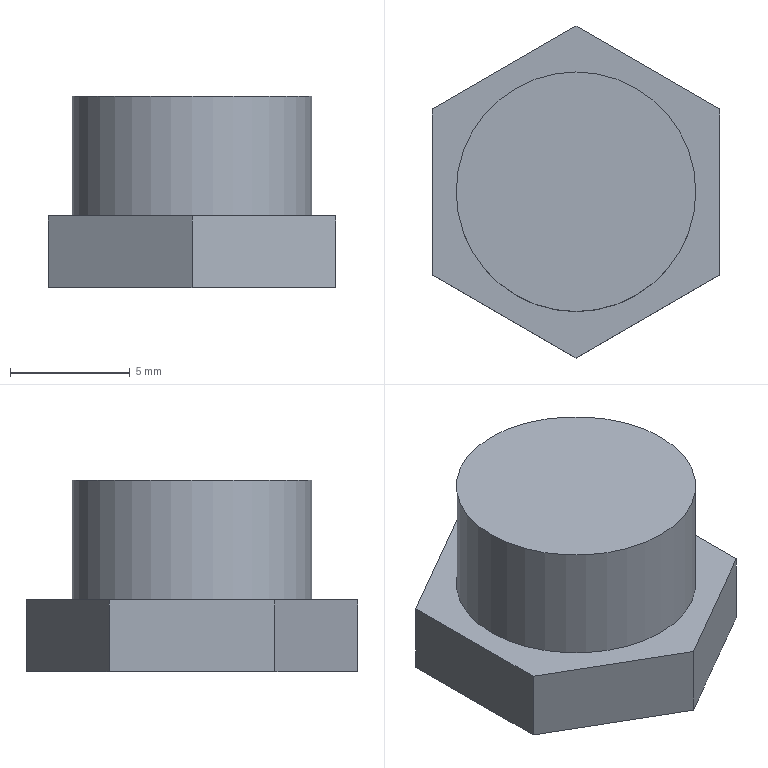Part | STEP file | 1-65.2 | 1 solid | 10 faces | box 12 x 13.856 x 8 mm | volume 766.822 mm3 | plane 9 | cylinder 1 | commonest cylinder face diameters 10 x1
STEP:
#1=CARTESIAN_POINT('',(0.,0.,0.));
#2=DIRECTION('',(0.,0.,1.));
#3=DIRECTION('',(1.,0.,0.));
#4=AXIS2_PLACEMENT_3D('',#1,#2,#3);
#5=CARTESIAN_POINT('',(-6.,-3.464,-3.));
#6=VERTEX_POINT('',#5);
#7=CARTESIAN_POINT('',(-6.,3.464,-3.));
#8=VERTEX_POINT('',#7);
#9=CARTESIAN_POINT('',(-6.,-3.464,-3.));
#10=DIRECTION('',(0.,1.,0.));
#11=VECTOR('',#10,1.);
#12=LINE('',#9,#11);
#13=CARTESIAN_POINT('',(0.9282,0.,-3.));
#14=DIRECTION('',(0.,0.,-1.));
#15=DIRECTION('',(1.,0.,0.));
#16=AXIS2_PLACEMENT_3D('',#13,#14,#15);
#17=PLANE('',#16);
#18=CARTESIAN_POINT('',(-6.928,3.464));
#19=DIRECTION('',(0.,-1.));
#20=VECTOR('',#19,1.);
#21=LINE('',#18,#20);
#22=(GEOMETRIC_REPRESENTATION_CONTEXT(2)PARAMETRIC_REPRESENTATION_CONTEXT()REPRESENTATION_CONTEXT('',''));
#23=DEFINITIONAL_REPRESENTATION('',(#21),#22);
#24=PCURVE('',#17,#23);
#25=CARTESIAN_POINT('',(-6.,0.,-1.5));
#26=DIRECTION('',(-1.,0.,0.));
#27=DIRECTION('',(0.,1.,0.));
#28=AXIS2_PLACEMENT_3D('',#25,#26,#27);
#29=PLANE('',#28);
#30=CARTESIAN_POINT('',(-3.464,1.5));
#31=DIRECTION('',(1.,0.));
#32=VECTOR('',#31,1.);
#33=LINE('',#30,#32);
#34=(GEOMETRIC_REPRESENTATION_CONTEXT(2)PARAMETRIC_REPRESENTATION_CONTEXT()REPRESENTATION_CONTEXT('',''));
#35=DEFINITIONAL_REPRESENTATION('',(#33),#34);
#36=PCURVE('',#29,#35);
#37=SURFACE_CURVE('',#12,(#24,#36),.PCURVE_S1.);
#38=EDGE_CURVE('',#6,#8,#37,.T.);
#39=ORIENTED_EDGE('',*,*,#38,.T.);
#40=CARTESIAN_POINT('',(0.,6.928,-3.));
#41=VERTEX_POINT('',#40);
#42=CARTESIAN_POINT('',(-6.,3.464,-3.));
#43=DIRECTION('',(0.866,0.5,0.));
#44=VECTOR('',#43,1.);
#45=LINE('',#42,#44);
#46=CARTESIAN_POINT('',(-6.928,-3.464));
#47=DIRECTION('',(0.866,-0.5));
#48=VECTOR('',#47,1.);
#49=LINE('',#46,#48);
#50=(GEOMETRIC_REPRESENTATION_CONTEXT(2)PARAMETRIC_REPRESENTATION_CONTEXT()REPRESENTATION_CONTEXT('',''));
#51=DEFINITIONAL_REPRESENTATION('',(#49),#50);
#52=PCURVE('',#17,#51);
#53=CARTESIAN_POINT('',(-3.,5.196,-1.5));
#54=DIRECTION('',(-0.5,0.866,0.));
#55=DIRECTION('',(0.866,0.5,0.));
#56=AXIS2_PLACEMENT_3D('',#53,#54,#55);
#57=PLANE('',#56);
#58=CARTESIAN_POINT('',(-3.464,1.5));
#59=DIRECTION('',(1.,0.));
#60=VECTOR('',#59,1.);
#61=LINE('',#58,#60);
#62=(GEOMETRIC_REPRESENTATION_CONTEXT(2)PARAMETRIC_REPRESENTATION_CONTEXT()REPRESENTATION_CONTEXT('',''));
#63=DEFINITIONAL_REPRESENTATION('',(#61),#62);
#64=PCURVE('',#57,#63);
#65=SURFACE_CURVE('',#45,(#52,#64),.PCURVE_S1.);
#66=EDGE_CURVE('',#8,#41,#65,.T.);
#67=ORIENTED_EDGE('',*,*,#66,.T.);
#68=CARTESIAN_POINT('',(6.,3.464,-3.));
#69=VERTEX_POINT('',#68);
#70=CARTESIAN_POINT('',(0.,6.928,-3.));
#71=DIRECTION('',(0.866,-0.5,0.));
#72=VECTOR('',#71,1.);
#73=LINE('',#70,#72);
#74=CARTESIAN_POINT('',(-0.9282,-6.928));
#75=DIRECTION('',(0.866,0.5));
#76=VECTOR('',#75,1.);
#77=LINE('',#74,#76);
#78=(GEOMETRIC_REPRESENTATION_CONTEXT(2)PARAMETRIC_REPRESENTATION_CONTEXT()REPRESENTATION_CONTEXT('',''));
#79=DEFINITIONAL_REPRESENTATION('',(#77),#78);
#80=PCURVE('',#17,#79);
#81=CARTESIAN_POINT('',(3.,5.196,-1.5));
#82=DIRECTION('',(0.5,0.866,0.));
#83=DIRECTION('',(0.866,-0.5,0.));
#84=AXIS2_PLACEMENT_3D('',#81,#82,#83);
#85=PLANE('',#84);
#86=CARTESIAN_POINT('',(-3.464,1.5));
#87=DIRECTION('',(1.,0.));
#88=VECTOR('',#87,1.);
#89=LINE('',#86,#88);
#90=(GEOMETRIC_REPRESENTATION_CONTEXT(2)PARAMETRIC_REPRESENTATION_CONTEXT()REPRESENTATION_CONTEXT('',''));
#91=DEFINITIONAL_REPRESENTATION('',(#89),#90);
#92=PCURVE('',#85,#91);
#93=SURFACE_CURVE('',#73,(#80,#92),.PCURVE_S1.);
#94=EDGE_CURVE('',#41,#69,#93,.T.);
#95=ORIENTED_EDGE('',*,*,#94,.T.);
#96=CARTESIAN_POINT('',(6.,-3.464,-3.));
#97=VERTEX_POINT('',#96);
#98=CARTESIAN_POINT('',(6.,3.464,-3.));
#99=DIRECTION('',(0.,-1.,0.));
#100=VECTOR('',#99,1.);
#101=LINE('',#98,#100);
#102=CARTESIAN_POINT('',(5.072,-3.464));
#103=DIRECTION('',(0.,1.));
#104=VECTOR('',#103,1.);
#105=LINE('',#102,#104);
#106=(GEOMETRIC_REPRESENTATION_CONTEXT(2)PARAMETRIC_REPRESENTATION_CONTEXT()REPRESENTATION_CONTEXT('',''));
#107=DEFINITIONAL_REPRESENTATION('',(#105),#106);
#108=PCURVE('',#17,#107);
#109=CARTESIAN_POINT('',(6.,0.,-1.5));
#110=DIRECTION('',(1.,0.,0.));
#111=DIRECTION('',(0.,-1.,0.));
#112=AXIS2_PLACEMENT_3D('',#109,#110,#111);
#113=PLANE('',#112);
#114=CARTESIAN_POINT('',(-3.464,1.5));
#115=DIRECTION('',(1.,0.));
#116=VECTOR('',#115,1.);
#117=LINE('',#114,#116);
#118=(GEOMETRIC_REPRESENTATION_CONTEXT(2)PARAMETRIC_REPRESENTATION_CONTEXT()REPRESENTATION_CONTEXT('',''));
#119=DEFINITIONAL_REPRESENTATION('',(#117),#118);
#120=PCURVE('',#113,#119);
#121=SURFACE_CURVE('',#101,(#108,#120),.PCURVE_S1.);
#122=EDGE_CURVE('',#69,#97,#121,.T.);
#123=ORIENTED_EDGE('',*,*,#122,.T.);
#124=CARTESIAN_POINT('',(0.,-6.928,-3.));
#125=VERTEX_POINT('',#124);
#126=CARTESIAN_POINT('',(6.,-3.464,-3.));
#127=DIRECTION('',(-0.866,-0.5,0.));
#128=VECTOR('',#127,1.);
#129=LINE('',#126,#128);
#130=CARTESIAN_POINT('',(5.072,3.464));
#131=DIRECTION('',(-0.866,0.5));
#132=VECTOR('',#131,1.);
#133=LINE('',#130,#132);
#134=(GEOMETRIC_REPRESENTATION_CONTEXT(2)PARAMETRIC_REPRESENTATION_CONTEXT()REPRESENTATION_CONTEXT('',''));
#135=DEFINITIONAL_REPRESENTATION('',(#133),#134);
#136=PCURVE('',#17,#135);
#137=CARTESIAN_POINT('',(3.,-5.196,-1.5));
#138=DIRECTION('',(0.5,-0.866,0.));
#139=DIRECTION('',(-0.866,-0.5,0.));
#140=AXIS2_PLACEMENT_3D('',#137,#138,#139);
#141=PLANE('',#140);
#142=CARTESIAN_POINT('',(-3.464,1.5));
#143=DIRECTION('',(1.,0.));
#144=VECTOR('',#143,1.);
#145=LINE('',#142,#144);
#146=(GEOMETRIC_REPRESENTATION_CONTEXT(2)PARAMETRIC_REPRESENTATION_CONTEXT()REPRESENTATION_CONTEXT('',''));
#147=DEFINITIONAL_REPRESENTATION('',(#145),#146);
#148=PCURVE('',#141,#147);
#149=SURFACE_CURVE('',#129,(#136,#148),.PCURVE_S1.);
#150=EDGE_CURVE('',#97,#125,#149,.T.);
#151=ORIENTED_EDGE('',*,*,#150,.T.);
#152=CARTESIAN_POINT('',(0.,-6.928,-3.));
#153=DIRECTION('',(-0.866,0.5,0.));
#154=VECTOR('',#153,1.);
#155=LINE('',#152,#154);
#156=CARTESIAN_POINT('',(-0.9282,6.928));
#157=DIRECTION('',(-0.866,-0.5));
#158=VECTOR('',#157,1.);
#159=LINE('',#156,#158);
#160=(GEOMETRIC_REPRESENTATION_CONTEXT(2)PARAMETRIC_REPRESENTATION_CONTEXT()REPRESENTATION_CONTEXT('',''));
#161=DEFINITIONAL_REPRESENTATION('',(#159),#160);
#162=PCURVE('',#17,#161);
#163=CARTESIAN_POINT('',(-3.,-5.196,-1.5));
#164=DIRECTION('',(-0.5,-0.866,0.));
#165=DIRECTION('',(-0.866,0.5,0.));
#166=AXIS2_PLACEMENT_3D('',#163,#164,#165);
#167=PLANE('',#166);
#168=CARTESIAN_POINT('',(-3.464,1.5));
#169=DIRECTION('',(1.,0.));
#170=VECTOR('',#169,1.);
#171=LINE('',#168,#170);
#172=(GEOMETRIC_REPRESENTATION_CONTEXT(2)PARAMETRIC_REPRESENTATION_CONTEXT()REPRESENTATION_CONTEXT('',''));
#173=DEFINITIONAL_REPRESENTATION('',(#171),#172);
#174=PCURVE('',#167,#173);
#175=SURFACE_CURVE('',#155,(#162,#174),.PCURVE_S1.);
#176=EDGE_CURVE('',#125,#6,#175,.T.);
#177=ORIENTED_EDGE('',*,*,#176,.T.);
#178=EDGE_LOOP('',(#39,#67,#95,#123,#151,#177));
#179=FACE_BOUND('',#178,.T.);
#180=ADVANCED_FACE('',(#179),#17,.T.);
#181=CARTESIAN_POINT('',(-6.,-3.464,0.));
#182=VERTEX_POINT('',#181);
#183=CARTESIAN_POINT('',(-6.,3.464,0.));
#184=VERTEX_POINT('',#183);
#185=CARTESIAN_POINT('',(-6.,-3.464,0.));
#186=DIRECTION('',(0.,1.,0.));
#187=VECTOR('',#186,1.);
#188=LINE('',#185,#187);
#189=CARTESIAN_POINT('',(-3.464,-1.5));
#190=DIRECTION('',(1.,0.));
#191=VECTOR('',#190,1.);
#192=LINE('',#189,#191);
#193=(GEOMETRIC_REPRESENTATION_CONTEXT(2)PARAMETRIC_REPRESENTATION_CONTEXT()REPRESENTATION_CONTEXT('',''));
#194=DEFINITIONAL_REPRESENTATION('',(#192),#193);
#195=PCURVE('',#29,#194);
#196=CARTESIAN_POINT('',(0.9282,0.,0.));
#197=DIRECTION('',(0.,0.,-1.));
#198=DIRECTION('',(1.,0.,0.));
#199=AXIS2_PLACEMENT_3D('',#196,#197,#198);
#200=PLANE('',#199);
#201=CARTESIAN_POINT('',(-6.928,3.464));
#202=DIRECTION('',(0.,-1.));
#203=VECTOR('',#202,1.);
#204=LINE('',#201,#203);
#205=(GEOMETRIC_REPRESENTATION_CONTEXT(2)PARAMETRIC_REPRESENTATION_CONTEXT()REPRESENTATION_CONTEXT('',''));
#206=DEFINITIONAL_REPRESENTATION('',(#204),#205);
#207=PCURVE('',#200,#206);
#208=SURFACE_CURVE('',#188,(#195,#207),.PCURVE_S1.);
#209=EDGE_CURVE('',#182,#184,#208,.T.);
#210=ORIENTED_EDGE('',*,*,#209,.T.);
#211=CARTESIAN_POINT('',(-6.,3.464,0.));
#212=DIRECTION('',(0.,0.,-1.));
#213=VECTOR('',#212,1.);
#214=LINE('',#211,#213);
#215=CARTESIAN_POINT('',(3.464,-1.5));
#216=DIRECTION('',(0.,1.));
#217=VECTOR('',#216,1.);
#218=LINE('',#215,#217);
#219=(GEOMETRIC_REPRESENTATION_CONTEXT(2)PARAMETRIC_REPRESENTATION_CONTEXT()REPRESENTATION_CONTEXT('',''));
#220=DEFINITIONAL_REPRESENTATION('',(#218),#219);
#221=PCURVE('',#29,#220);
#222=CARTESIAN_POINT('',(-3.464,-1.5));
#223=DIRECTION('',(0.,1.));
#224=VECTOR('',#223,1.);
#225=LINE('',#222,#224);
#226=(GEOMETRIC_REPRESENTATION_CONTEXT(2)PARAMETRIC_REPRESENTATION_CONTEXT()REPRESENTATION_CONTEXT('',''));
#227=DEFINITIONAL_REPRESENTATION('',(#225),#226);
#228=PCURVE('',#57,#227);
#229=SURFACE_CURVE('',#214,(#221,#228),.PCURVE_S1.);
#230=EDGE_CURVE('',#184,#8,#229,.T.);
#231=ORIENTED_EDGE('',*,*,#230,.T.);
#232=ORIENTED_EDGE('',*,*,#38,.F.);
#233=CARTESIAN_POINT('',(-6.,-3.464,0.));
#234=DIRECTION('',(0.,0.,-1.));
#235=VECTOR('',#234,1.);
#236=LINE('',#233,#235);
#237=CARTESIAN_POINT('',(-3.464,-1.5));
#238=DIRECTION('',(0.,1.));
#239=VECTOR('',#238,1.);
#240=LINE('',#237,#239);
#241=(GEOMETRIC_REPRESENTATION_CONTEXT(2)PARAMETRIC_REPRESENTATION_CONTEXT()REPRESENTATION_CONTEXT('',''));
#242=DEFINITIONAL_REPRESENTATION('',(#240),#241);
#243=PCURVE('',#29,#242);
#244=CARTESIAN_POINT('',(3.464,-1.5));
#245=DIRECTION('',(0.,1.));
#246=VECTOR('',#245,1.);
#247=LINE('',#244,#246);
#248=(GEOMETRIC_REPRESENTATION_CONTEXT(2)PARAMETRIC_REPRESENTATION_CONTEXT()REPRESENTATION_CONTEXT('',''));
#249=DEFINITIONAL_REPRESENTATION('',(#247),#248);
#250=PCURVE('',#167,#249);
#251=SURFACE_CURVE('',#236,(#243,#250),.PCURVE_S1.);
#252=EDGE_CURVE('',#182,#6,#251,.T.);
#253=ORIENTED_EDGE('',*,*,#252,.F.);
#254=EDGE_LOOP('',(#210,#231,#232,#253));
#255=FACE_BOUND('',#254,.T.);
#256=ADVANCED_FACE('',(#255),#29,.T.);
#257=CARTESIAN_POINT('',(0.,6.928,0.));
#258=VERTEX_POINT('',#257);
#259=CARTESIAN_POINT('',(-6.,3.464,0.));
#260=DIRECTION('',(0.866,0.5,0.));
#261=VECTOR('',#260,1.);
#262=LINE('',#259,#261);
#263=CARTESIAN_POINT('',(-3.464,-1.5));
#264=DIRECTION('',(1.,0.));
#265=VECTOR('',#264,1.);
#266=LINE('',#263,#265);
#267=(GEOMETRIC_REPRESENTATION_CONTEXT(2)PARAMETRIC_REPRESENTATION_CONTEXT()REPRESENTATION_CONTEXT('',''));
#268=DEFINITIONAL_REPRESENTATION('',(#266),#267);
#269=PCURVE('',#57,#268);
#270=CARTESIAN_POINT('',(-6.928,-3.464));
#271=DIRECTION('',(0.866,-0.5));
#272=VECTOR('',#271,1.);
#273=LINE('',#270,#272);
#274=(GEOMETRIC_REPRESENTATION_CONTEXT(2)PARAMETRIC_REPRESENTATION_CONTEXT()REPRESENTATION_CONTEXT('',''));
#275=DEFINITIONAL_REPRESENTATION('',(#273),#274);
#276=PCURVE('',#200,#275);
#277=SURFACE_CURVE('',#262,(#269,#276),.PCURVE_S1.);
#278=EDGE_CURVE('',#184,#258,#277,.T.);
#279=ORIENTED_EDGE('',*,*,#278,.T.);
#280=CARTESIAN_POINT('',(0.,6.928,0.));
#281=DIRECTION('',(0.,0.,-1.));
#282=VECTOR('',#281,1.);
#283=LINE('',#280,#282);
#284=CARTESIAN_POINT('',(3.464,-1.5));
#285=DIRECTION('',(0.,1.));
#286=VECTOR('',#285,1.);
#287=LINE('',#284,#286);
#288=(GEOMETRIC_REPRESENTATION_CONTEXT(2)PARAMETRIC_REPRESENTATION_CONTEXT()REPRESENTATION_CONTEXT('',''));
#289=DEFINITIONAL_REPRESENTATION('',(#287),#288);
#290=PCURVE('',#57,#289);
#291=CARTESIAN_POINT('',(-3.464,-1.5));
#292=DIRECTION('',(0.,1.));
#293=VECTOR('',#292,1.);
#294=LINE('',#291,#293);
#295=(GEOMETRIC_REPRESENTATION_CONTEXT(2)PARAMETRIC_REPRESENTATION_CONTEXT()REPRESENTATION_CONTEXT('',''));
#296=DEFINITIONAL_REPRESENTATION('',(#294),#295);
#297=PCURVE('',#85,#296);
#298=SURFACE_CURVE('',#283,(#290,#297),.PCURVE_S1.);
#299=EDGE_CURVE('',#258,#41,#298,.T.);
#300=ORIENTED_EDGE('',*,*,#299,.T.);
#301=ORIENTED_EDGE('',*,*,#66,.F.);
#302=ORIENTED_EDGE('',*,*,#230,.F.);
#303=EDGE_LOOP('',(#279,#300,#301,#302));
#304=FACE_BOUND('',#303,.T.);
#305=ADVANCED_FACE('',(#304),#57,.T.);
#306=CARTESIAN_POINT('',(6.,3.464,0.));
#307=VERTEX_POINT('',#306);
#308=CARTESIAN_POINT('',(0.,6.928,0.));
#309=DIRECTION('',(0.866,-0.5,0.));
#310=VECTOR('',#309,1.);
#311=LINE('',#308,#310);
#312=CARTESIAN_POINT('',(-3.464,-1.5));
#313=DIRECTION('',(1.,0.));
#314=VECTOR('',#313,1.);
#315=LINE('',#312,#314);
#316=(GEOMETRIC_REPRESENTATION_CONTEXT(2)PARAMETRIC_REPRESENTATION_CONTEXT()REPRESENTATION_CONTEXT('',''));
#317=DEFINITIONAL_REPRESENTATION('',(#315),#316);
#318=PCURVE('',#85,#317);
#319=CARTESIAN_POINT('',(-0.9282,-6.928));
#320=DIRECTION('',(0.866,0.5));
#321=VECTOR('',#320,1.);
#322=LINE('',#319,#321);
#323=(GEOMETRIC_REPRESENTATION_CONTEXT(2)PARAMETRIC_REPRESENTATION_CONTEXT()REPRESENTATION_CONTEXT('',''));
#324=DEFINITIONAL_REPRESENTATION('',(#322),#323);
#325=PCURVE('',#200,#324);
#326=SURFACE_CURVE('',#311,(#318,#325),.PCURVE_S1.);
#327=EDGE_CURVE('',#258,#307,#326,.T.);
#328=ORIENTED_EDGE('',*,*,#327,.T.);
#329=CARTESIAN_POINT('',(6.,3.464,0.));
#330=DIRECTION('',(0.,0.,-1.));
#331=VECTOR('',#330,1.);
#332=LINE('',#329,#331);
#333=CARTESIAN_POINT('',(3.464,-1.5));
#334=DIRECTION('',(0.,1.));
#335=VECTOR('',#334,1.);
#336=LINE('',#333,#335);
#337=(GEOMETRIC_REPRESENTATION_CONTEXT(2)PARAMETRIC_REPRESENTATION_CONTEXT()REPRESENTATION_CONTEXT('',''));
#338=DEFINITIONAL_REPRESENTATION('',(#336),#337);
#339=PCURVE('',#85,#338);
#340=CARTESIAN_POINT('',(-3.464,-1.5));
#341=DIRECTION('',(0.,1.));
#342=VECTOR('',#341,1.);
#343=LINE('',#340,#342);
#344=(GEOMETRIC_REPRESENTATION_CONTEXT(2)PARAMETRIC_REPRESENTATION_CONTEXT()REPRESENTATION_CONTEXT('',''));
#345=DEFINITIONAL_REPRESENTATION('',(#343),#344);
#346=PCURVE('',#113,#345);
#347=SURFACE_CURVE('',#332,(#339,#346),.PCURVE_S1.);
#348=EDGE_CURVE('',#307,#69,#347,.T.);
#349=ORIENTED_EDGE('',*,*,#348,.T.);
#350=ORIENTED_EDGE('',*,*,#94,.F.);
#351=ORIENTED_EDGE('',*,*,#299,.F.);
#352=EDGE_LOOP('',(#328,#349,#350,#351));
#353=FACE_BOUND('',#352,.T.);
#354=ADVANCED_FACE('',(#353),#85,.T.);
#355=CARTESIAN_POINT('',(6.,-3.464,0.));
#356=VERTEX_POINT('',#355);
#357=CARTESIAN_POINT('',(6.,3.464,0.));
#358=DIRECTION('',(0.,-1.,0.));
#359=VECTOR('',#358,1.);
#360=LINE('',#357,#359);
#361=CARTESIAN_POINT('',(-3.464,-1.5));
#362=DIRECTION('',(1.,0.));
#363=VECTOR('',#362,1.);
#364=LINE('',#361,#363);
#365=(GEOMETRIC_REPRESENTATION_CONTEXT(2)PARAMETRIC_REPRESENTATION_CONTEXT()REPRESENTATION_CONTEXT('',''));
#366=DEFINITIONAL_REPRESENTATION('',(#364),#365);
#367=PCURVE('',#113,#366);
#368=CARTESIAN_POINT('',(5.072,-3.464));
#369=DIRECTION('',(0.,1.));
#370=VECTOR('',#369,1.);
#371=LINE('',#368,#370);
#372=(GEOMETRIC_REPRESENTATION_CONTEXT(2)PARAMETRIC_REPRESENTATION_CONTEXT()REPRESENTATION_CONTEXT('',''));
#373=DEFINITIONAL_REPRESENTATION('',(#371),#372);
#374=PCURVE('',#200,#373);
#375=SURFACE_CURVE('',#360,(#367,#374),.PCURVE_S1.);
#376=EDGE_CURVE('',#307,#356,#375,.T.);
#377=ORIENTED_EDGE('',*,*,#376,.T.);
#378=CARTESIAN_POINT('',(6.,-3.464,0.));
#379=DIRECTION('',(0.,0.,-1.));
#380=VECTOR('',#379,1.);
#381=LINE('',#378,#380);
#382=CARTESIAN_POINT('',(3.464,-1.5));
#383=DIRECTION('',(0.,1.));
#384=VECTOR('',#383,1.);
#385=LINE('',#382,#384);
#386=(GEOMETRIC_REPRESENTATION_CONTEXT(2)PARAMETRIC_REPRESENTATION_CONTEXT()REPRESENTATION_CONTEXT('',''));
#387=DEFINITIONAL_REPRESENTATION('',(#385),#386);
#388=PCURVE('',#113,#387);
#389=CARTESIAN_POINT('',(-3.464,-1.5));
#390=DIRECTION('',(0.,1.));
#391=VECTOR('',#390,1.);
#392=LINE('',#389,#391);
#393=(GEOMETRIC_REPRESENTATION_CONTEXT(2)PARAMETRIC_REPRESENTATION_CONTEXT()REPRESENTATION_CONTEXT('',''));
#394=DEFINITIONAL_REPRESENTATION('',(#392),#393);
#395=PCURVE('',#141,#394);
#396=SURFACE_CURVE('',#381,(#388,#395),.PCURVE_S1.);
#397=EDGE_CURVE('',#356,#97,#396,.T.);
#398=ORIENTED_EDGE('',*,*,#397,.T.);
#399=ORIENTED_EDGE('',*,*,#122,.F.);
#400=ORIENTED_EDGE('',*,*,#348,.F.);
#401=EDGE_LOOP('',(#377,#398,#399,#400));
#402=FACE_BOUND('',#401,.T.);
#403=ADVANCED_FACE('',(#402),#113,.T.);
#404=CARTESIAN_POINT('',(0.,-6.928,0.));
#405=VERTEX_POINT('',#404);
#406=CARTESIAN_POINT('',(6.,-3.464,0.));
#407=DIRECTION('',(-0.866,-0.5,0.));
#408=VECTOR('',#407,1.);
#409=LINE('',#406,#408);
#410=CARTESIAN_POINT('',(-3.464,-1.5));
#411=DIRECTION('',(1.,0.));
#412=VECTOR('',#411,1.);
#413=LINE('',#410,#412);
#414=(GEOMETRIC_REPRESENTATION_CONTEXT(2)PARAMETRIC_REPRESENTATION_CONTEXT()REPRESENTATION_CONTEXT('',''));
#415=DEFINITIONAL_REPRESENTATION('',(#413),#414);
#416=PCURVE('',#141,#415);
#417=CARTESIAN_POINT('',(5.072,3.464));
#418=DIRECTION('',(-0.866,0.5));
#419=VECTOR('',#418,1.);
#420=LINE('',#417,#419);
#421=(GEOMETRIC_REPRESENTATION_CONTEXT(2)PARAMETRIC_REPRESENTATION_CONTEXT()REPRESENTATION_CONTEXT('',''));
#422=DEFINITIONAL_REPRESENTATION('',(#420),#421);
#423=PCURVE('',#200,#422);
#424=SURFACE_CURVE('',#409,(#416,#423),.PCURVE_S1.);
#425=EDGE_CURVE('',#356,#405,#424,.T.);
#426=ORIENTED_EDGE('',*,*,#425,.T.);
#427=CARTESIAN_POINT('',(0.,-6.928,0.));
#428=DIRECTION('',(0.,0.,-1.));
#429=VECTOR('',#428,1.);
#430=LINE('',#427,#429);
#431=CARTESIAN_POINT('',(3.464,-1.5));
#432=DIRECTION('',(0.,1.));
#433=VECTOR('',#432,1.);
#434=LINE('',#431,#433);
#435=(GEOMETRIC_REPRESENTATION_CONTEXT(2)PARAMETRIC_REPRESENTATION_CONTEXT()REPRESENTATION_CONTEXT('',''));
#436=DEFINITIONAL_REPRESENTATION('',(#434),#435);
#437=PCURVE('',#141,#436);
#438=CARTESIAN_POINT('',(-3.464,-1.5));
#439=DIRECTION('',(0.,1.));
#440=VECTOR('',#439,1.);
#441=LINE('',#438,#440);
#442=(GEOMETRIC_REPRESENTATION_CONTEXT(2)PARAMETRIC_REPRESENTATION_CONTEXT()REPRESENTATION_CONTEXT('',''));
#443=DEFINITIONAL_REPRESENTATION('',(#441),#442);
#444=PCURVE('',#167,#443);
#445=SURFACE_CURVE('',#430,(#437,#444),.PCURVE_S1.);
#446=EDGE_CURVE('',#405,#125,#445,.T.);
#447=ORIENTED_EDGE('',*,*,#446,.T.);
#448=ORIENTED_EDGE('',*,*,#150,.F.);
#449=ORIENTED_EDGE('',*,*,#397,.F.);
#450=EDGE_LOOP('',(#426,#447,#448,#449));
#451=FACE_BOUND('',#450,.T.);
#452=ADVANCED_FACE('',(#451),#141,.T.);
#453=CARTESIAN_POINT('',(0.,-6.928,0.));
#454=DIRECTION('',(-0.866,0.5,0.));
#455=VECTOR('',#454,1.);
#456=LINE('',#453,#455);
#457=CARTESIAN_POINT('',(-3.464,-1.5));
#458=DIRECTION('',(1.,0.));
#459=VECTOR('',#458,1.);
#460=LINE('',#457,#459);
#461=(GEOMETRIC_REPRESENTATION_CONTEXT(2)PARAMETRIC_REPRESENTATION_CONTEXT()REPRESENTATION_CONTEXT('',''));
#462=DEFINITIONAL_REPRESENTATION('',(#460),#461);
#463=PCURVE('',#167,#462);
#464=CARTESIAN_POINT('',(-0.9282,6.928));
#465=DIRECTION('',(-0.866,-0.5));
#466=VECTOR('',#465,1.);
#467=LINE('',#464,#466);
#468=(GEOMETRIC_REPRESENTATION_CONTEXT(2)PARAMETRIC_REPRESENTATION_CONTEXT()REPRESENTATION_CONTEXT('',''));
#469=DEFINITIONAL_REPRESENTATION('',(#467),#468);
#470=PCURVE('',#200,#469);
#471=SURFACE_CURVE('',#456,(#463,#470),.PCURVE_S1.);
#472=EDGE_CURVE('',#405,#182,#471,.T.);
#473=ORIENTED_EDGE('',*,*,#472,.T.);
#474=ORIENTED_EDGE('',*,*,#252,.T.);
#475=ORIENTED_EDGE('',*,*,#176,.F.);
#476=ORIENTED_EDGE('',*,*,#446,.F.);
#477=EDGE_LOOP('',(#473,#474,#475,#476));
#478=FACE_BOUND('',#477,.T.);
#479=ADVANCED_FACE('',(#478),#167,.T.);
#480=ORIENTED_EDGE('',*,*,#209,.T.);
#481=ORIENTED_EDGE('',*,*,#278,.T.);
#482=ORIENTED_EDGE('',*,*,#327,.T.);
#483=ORIENTED_EDGE('',*,*,#376,.T.);
#484=ORIENTED_EDGE('',*,*,#425,.T.);
#485=ORIENTED_EDGE('',*,*,#472,.T.);
#486=EDGE_LOOP('',(#480,#481,#482,#483,#484,#485));
#487=FACE_BOUND('',#486,.F.);
#488=CARTESIAN_POINT('',(0.,5.,0.));
#489=VERTEX_POINT('',#488);
#490=CARTESIAN_POINT('',(0.,0.,0.));
#491=DIRECTION('',(0.,0.,1.));
#492=DIRECTION('',(0.,1.,0.));
#493=AXIS2_PLACEMENT_3D('',#490,#491,#492);
#494=CIRCLE('',#493,5.);
#495=CARTESIAN_POINT('',(-0.9282,-5.));
#496=CARTESIAN_POINT('',(-9.588,-5.));
#497=CARTESIAN_POINT('',(-5.258,2.5));
#498=CARTESIAN_POINT('',(-0.9282,10.));
#499=CARTESIAN_POINT('',(3.402,2.5));
#500=CARTESIAN_POINT('',(7.732,-5.));
#501=CARTESIAN_POINT('',(-0.9282,-5.));
#502=(BOUNDED_CURVE()B_SPLINE_CURVE(2,(#495,#496,#497,#498,#499,#500,#501),.UNSPECIFIED.,.T.,.F.)B_SPLINE_CURVE_WITH_KNOTS((1,2,2,2,2,1),(-2.094,0.,2.094,4.189,6.283,8.378),.UNSPECIFIED.)CURVE()GEOMETRIC_REPRESENTATION_ITEM()RATIONAL_B_SPLINE_CURVE((1.,0.5,1.,0.5,1.,0.5,1.))REPRESENTATION_ITEM(''));
#503=(GEOMETRIC_REPRESENTATION_CONTEXT(2)PARAMETRIC_REPRESENTATION_CONTEXT()REPRESENTATION_CONTEXT('',''));
#504=DEFINITIONAL_REPRESENTATION('',(#502),#503);
#505=PCURVE('',#200,#504);
#506=CARTESIAN_POINT('',(0.,0.,0.));
#507=DIRECTION('',(0.,0.,1.));
#508=DIRECTION('',(0.,1.,0.));
#509=AXIS2_PLACEMENT_3D('',#506,#507,#508);
#510=CYLINDRICAL_SURFACE('',#509,5.);
#511=CARTESIAN_POINT('',(0.,0.));
#512=DIRECTION('',(1.,0.));
#513=VECTOR('',#512,1.);
#514=LINE('',#511,#513);
#515=(GEOMETRIC_REPRESENTATION_CONTEXT(2)PARAMETRIC_REPRESENTATION_CONTEXT()REPRESENTATION_CONTEXT('',''));
#516=DEFINITIONAL_REPRESENTATION('',(#514),#515);
#517=PCURVE('',#510,#516);
#518=SURFACE_CURVE('',#494,(#505,#517),.PCURVE_S1.);
#519=EDGE_CURVE('',#489,#489,#518,.T.);
#520=ORIENTED_EDGE('',*,*,#519,.T.);
#521=EDGE_LOOP('',(#520));
#522=FACE_BOUND('',#521,.F.);
#523=ADVANCED_FACE('',(#487,#522),#200,.F.);
#524=ORIENTED_EDGE('',*,*,#519,.T.);
#525=CARTESIAN_POINT('',(0.,5.,5.));
#526=VERTEX_POINT('',#525);
#527=CARTESIAN_POINT('',(0.,5.,0.));
#528=DIRECTION('',(0.,0.,1.));
#529=VECTOR('',#528,1.);
#530=LINE('',#527,#529);
#531=CARTESIAN_POINT('',(6.283,0.));
#532=DIRECTION('',(0.,1.));
#533=VECTOR('',#532,1.);
#534=LINE('',#531,#533);
#535=(GEOMETRIC_REPRESENTATION_CONTEXT(2)PARAMETRIC_REPRESENTATION_CONTEXT()REPRESENTATION_CONTEXT('',''));
#536=DEFINITIONAL_REPRESENTATION('',(#534),#535);
#537=PCURVE('',#510,#536);
#538=CARTESIAN_POINT('',(0.,0.));
#539=DIRECTION('',(0.,1.));
#540=VECTOR('',#539,1.);
#541=LINE('',#538,#540);
#542=(GEOMETRIC_REPRESENTATION_CONTEXT(2)PARAMETRIC_REPRESENTATION_CONTEXT()REPRESENTATION_CONTEXT('',''));
#543=DEFINITIONAL_REPRESENTATION('',(#541),#542);
#544=PCURVE('',#510,#543);
#545=SEAM_CURVE('',#530,(#537,#544),.PCURVE_S1.);
#546=EDGE_CURVE('',#489,#526,#545,.T.);
#547=ORIENTED_EDGE('',*,*,#546,.T.);
#548=CARTESIAN_POINT('',(0.,0.,5.));
#549=DIRECTION('',(0.,0.,1.));
#550=DIRECTION('',(0.,1.,0.));
#551=AXIS2_PLACEMENT_3D('',#548,#549,#550);
#552=CIRCLE('',#551,5.);
#553=CARTESIAN_POINT('',(0.,5.));
#554=DIRECTION('',(1.,0.));
#555=VECTOR('',#554,1.);
#556=LINE('',#553,#555);
#557=(GEOMETRIC_REPRESENTATION_CONTEXT(2)PARAMETRIC_REPRESENTATION_CONTEXT()REPRESENTATION_CONTEXT('',''));
#558=DEFINITIONAL_REPRESENTATION('',(#556),#557);
#559=PCURVE('',#510,#558);
#560=CARTESIAN_POINT('',(0.,-1.34,5.));
#561=DIRECTION('',(0.,0.,1.));
#562=DIRECTION('',(1.,0.,0.));
#563=AXIS2_PLACEMENT_3D('',#560,#561,#562);
#564=PLANE('',#563);
#565=CARTESIAN_POINT('',(0.,1.34));
#566=DIRECTION('',(0.,1.));
#567=AXIS2_PLACEMENT_2D('',#565,#566);
#568=CIRCLE('',#567,5.);
#569=(GEOMETRIC_REPRESENTATION_CONTEXT(2)PARAMETRIC_REPRESENTATION_CONTEXT()REPRESENTATION_CONTEXT('',''));
#570=DEFINITIONAL_REPRESENTATION('',(#568),#569);
#571=PCURVE('',#564,#570);
#572=SURFACE_CURVE('',#552,(#559,#571),.PCURVE_S1.);
#573=EDGE_CURVE('',#526,#526,#572,.T.);
#574=ORIENTED_EDGE('',*,*,#573,.F.);
#575=ORIENTED_EDGE('',*,*,#546,.F.);
#576=EDGE_LOOP('',(#524,#547,#574,#575));
#577=FACE_BOUND('',#576,.T.);
#578=ADVANCED_FACE('',(#577),#510,.T.);
#579=ORIENTED_EDGE('',*,*,#573,.T.);
#580=EDGE_LOOP('',(#579));
#581=FACE_BOUND('',#580,.T.);
#582=ADVANCED_FACE('',(#581),#564,.T.);
#583=CLOSED_SHELL('',(#180,#256,#305,#354,#403,#452,#479,#523,#578,#582));
#584=MANIFOLD_SOLID_BREP('',#583);
#585=(LENGTH_UNIT()NAMED_UNIT(*)SI_UNIT(.MILLI.,.METRE.));
#586=UNCERTAINTY_MEASURE_WITH_UNIT(LENGTH_MEASURE(0.0000001),#585,'','');
#587=(NAMED_UNIT(*)PLANE_ANGLE_UNIT()SI_UNIT($,.RADIAN.));
#588=(NAMED_UNIT(*)SI_UNIT($,.STERADIAN.)SOLID_ANGLE_UNIT());
#589=(GEOMETRIC_REPRESENTATION_CONTEXT(3)GLOBAL_UNCERTAINTY_ASSIGNED_CONTEXT((#586))GLOBAL_UNIT_ASSIGNED_CONTEXT((#585,#587,#588))REPRESENTATION_CONTEXT('',''));
#590=ADVANCED_BREP_SHAPE_REPRESENTATION('',(#4,#584),#589);